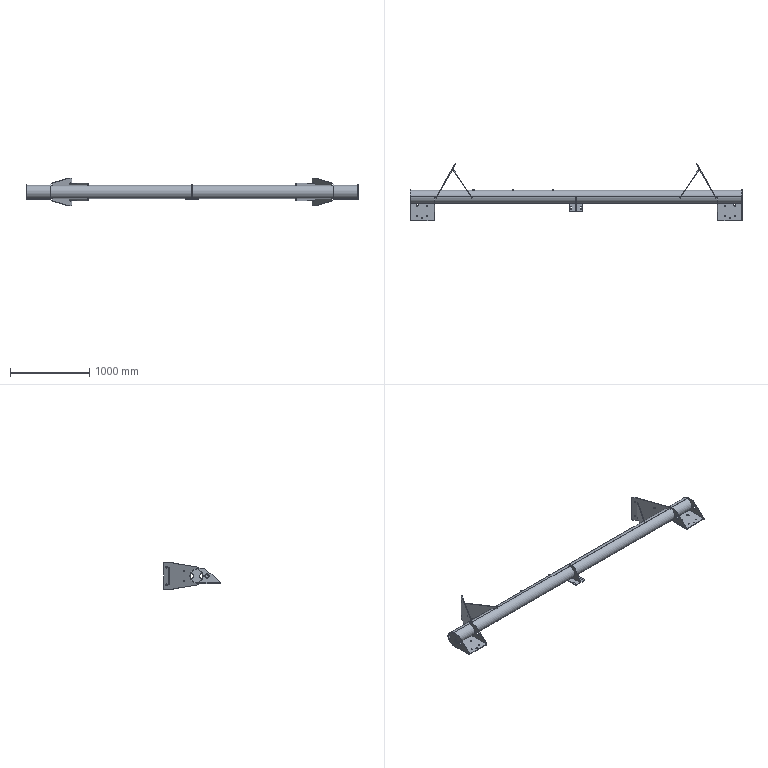Part | SolidWorks | features ICE 11, Cut 3, Fillet 3, BossThin 2, Extrusion 1, MirrorSolid 1 | 17 solids | 273 faces | box 4180 x 717.634 x 350 mm | volume 12364755 mm3 | plane 148 | cylinder 117 | spline 8 | commonest cylinder face diameters 6 x18 10 x18 13 x18 18 x16 20 x14 11 x8